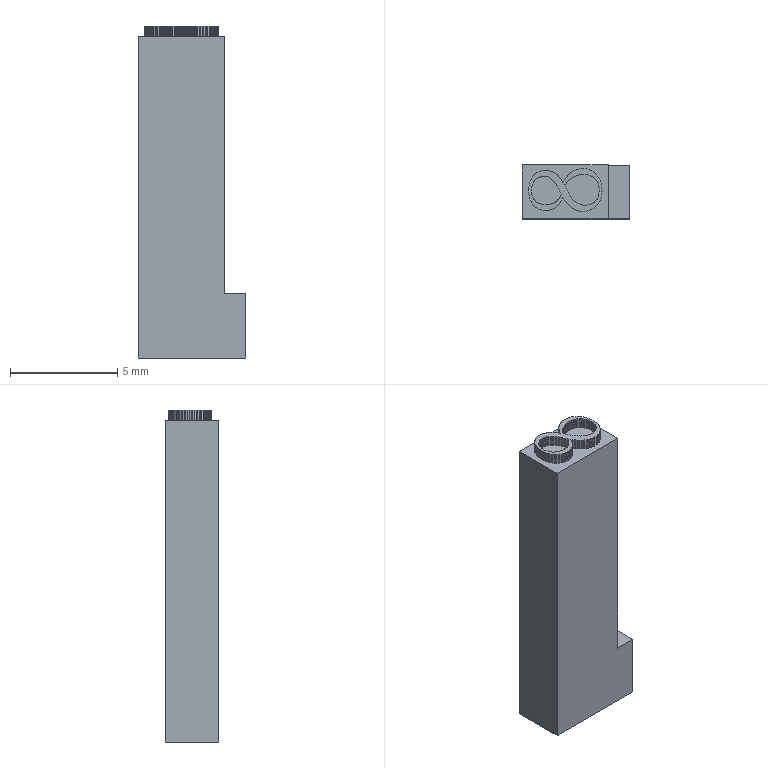Part | NX | features DIE-30 2 | 1 solid | 331 faces | box 5 x 2.5 x 15.5 mm | volume 158.632 mm3 | plane 331